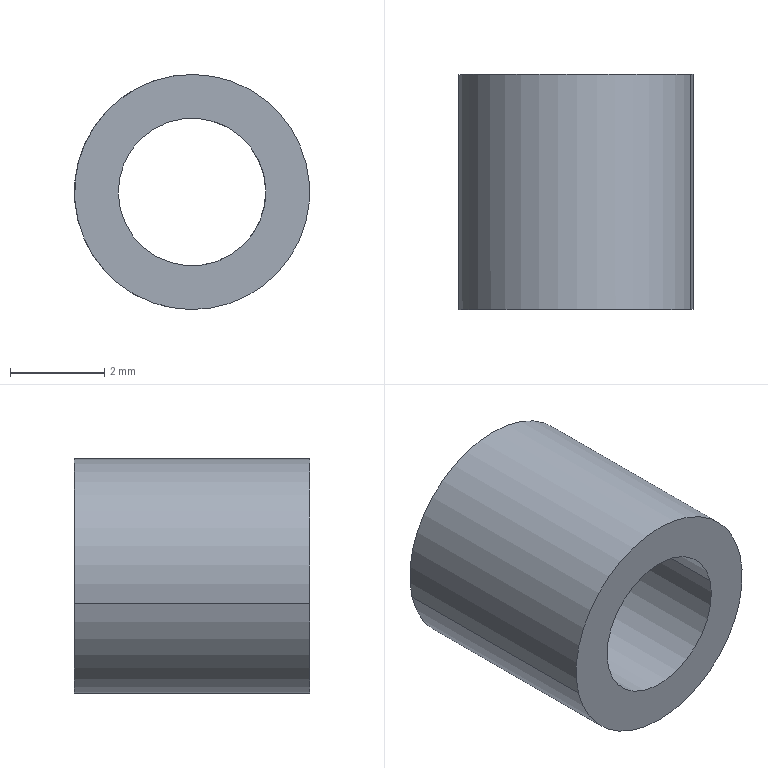Part | SolidWorks | features BaseBody 1 | 1 solid | 6 faces | box 5.005 x 5.005 x 5 mm | volume 59.456 mm3 | cylinder 4 | plane 2 | commonest cylinder face diameters 3.14 x2 5 x2
STEP:
#1=CARTESIAN_POINT('',(343.446,427.466,107.288));
#2=VERTEX_POINT('',#1);
#3=CARTESIAN_POINT('',(340.393,427.463,106.551));
#4=VERTEX_POINT('',#3);
#5=CARTESIAN_POINT('',(341.92,427.464,106.919));
#6=DIRECTION('',(0.0009599,-1.,0.));
#7=DIRECTION('',(-0.9721,-0.0009331,-0.2347));
#8=AXIS2_PLACEMENT_3D('',#5,#6,#7);
#9=CIRCLE('',#8,1.57);
#10=EDGE_CURVE('',#2,#4,#9,.T.);
#11=ORIENTED_EDGE('',*,*,#10,.F.);
#12=CARTESIAN_POINT('',(343.451,422.466,107.288));
#13=VERTEX_POINT('',#12);
#14=CARTESIAN_POINT('',(343.446,427.466,107.288));
#15=DIRECTION('',(0.0009599,-1.,0.));
#16=VECTOR('',#15,1000.);
#17=LINE('',#14,#16);
#18=EDGE_CURVE('',#2,#13,#17,.T.);
#19=ORIENTED_EDGE('',*,*,#18,.T.);
#20=CARTESIAN_POINT('',(340.398,422.463,106.551));
#21=VERTEX_POINT('',#20);
#22=CARTESIAN_POINT('',(341.924,422.464,106.919));
#23=DIRECTION('',(-0.0009599,1.,0.));
#24=DIRECTION('',(0.9721,0.0009331,0.2347));
#25=AXIS2_PLACEMENT_3D('',#22,#23,#24);
#26=CIRCLE('',#25,1.57);
#27=EDGE_CURVE('',#21,#13,#26,.T.);
#28=ORIENTED_EDGE('',*,*,#27,.F.);
#29=CARTESIAN_POINT('',(340.393,427.463,106.551));
#30=DIRECTION('',(0.0009599,-1.,0.));
#31=VECTOR('',#30,1000.);
#32=LINE('',#29,#31);
#33=EDGE_CURVE('',#4,#21,#32,.T.);
#34=ORIENTED_EDGE('',*,*,#33,.F.);
#35=EDGE_LOOP('',(#11,#19,#28,#34));
#36=FACE_OUTER_BOUND('',#35,.T.);
#37=CARTESIAN_POINT('',(341.92,427.464,106.919));
#38=DIRECTION('',(0.0009599,-1.,0.));
#39=DIRECTION('',(-0.9721,-0.0009331,-0.2347));
#40=AXIS2_PLACEMENT_3D('',#37,#38,#39);
#41=CYLINDRICAL_SURFACE('',#40,1.57);
#42=ADVANCED_FACE('',(#36),#41,.F.);
#43=CARTESIAN_POINT('',(344.35,427.466,107.506));
#44=VERTEX_POINT('',#43);
#45=CARTESIAN_POINT('',(339.489,427.462,106.332));
#46=VERTEX_POINT('',#45);
#47=CARTESIAN_POINT('',(341.92,427.464,106.919));
#48=DIRECTION('',(-0.0009599,1.,0.));
#49=DIRECTION('',(0.9721,0.0009331,0.2347));
#50=AXIS2_PLACEMENT_3D('',#47,#48,#49);
#51=CIRCLE('',#50,2.5);
#52=EDGE_CURVE('',#44,#46,#51,.T.);
#53=ORIENTED_EDGE('',*,*,#52,.F.);
#54=CARTESIAN_POINT('',(344.355,422.466,107.506));
#55=VERTEX_POINT('',#54);
#56=CARTESIAN_POINT('',(344.35,427.466,107.506));
#57=DIRECTION('',(0.0009599,-1.,0.));
#58=VECTOR('',#57,1000.);
#59=LINE('',#56,#58);
#60=EDGE_CURVE('',#44,#55,#59,.T.);
#61=ORIENTED_EDGE('',*,*,#60,.T.);
#62=CARTESIAN_POINT('',(339.494,422.462,106.332));
#63=VERTEX_POINT('',#62);
#64=CARTESIAN_POINT('',(341.924,422.464,106.919));
#65=DIRECTION('',(0.0009599,-1.,0.));
#66=DIRECTION('',(0.9721,0.0009331,0.2347));
#67=AXIS2_PLACEMENT_3D('',#64,#65,#66);
#68=CIRCLE('',#67,2.5);
#69=EDGE_CURVE('',#63,#55,#68,.T.);
#70=ORIENTED_EDGE('',*,*,#69,.F.);
#71=CARTESIAN_POINT('',(339.489,427.462,106.332));
#72=DIRECTION('',(0.0009599,-1.,0.));
#73=VECTOR('',#72,1000.);
#74=LINE('',#71,#73);
#75=EDGE_CURVE('',#46,#63,#74,.T.);
#76=ORIENTED_EDGE('',*,*,#75,.F.);
#77=EDGE_LOOP('',(#53,#61,#70,#76));
#78=FACE_OUTER_BOUND('',#77,.T.);
#79=CARTESIAN_POINT('',(341.92,427.464,106.919));
#80=DIRECTION('',(0.0009599,-1.,0.));
#81=DIRECTION('',(-0.9721,-0.0009331,-0.2347));
#82=AXIS2_PLACEMENT_3D('',#79,#80,#81);
#83=CYLINDRICAL_SURFACE('',#82,2.5);
#84=ADVANCED_FACE('',(#78),#83,.T.);
#85=ORIENTED_EDGE('',*,*,#27,.T.);
#86=CARTESIAN_POINT('',(341.924,422.464,106.919));
#87=DIRECTION('',(-0.0009599,1.,0.));
#88=DIRECTION('',(0.9721,0.0009331,0.2347));
#89=AXIS2_PLACEMENT_3D('',#86,#87,#88);
#90=CIRCLE('',#89,1.57);
#91=EDGE_CURVE('',#13,#21,#90,.T.);
#92=ORIENTED_EDGE('',*,*,#91,.T.);
#93=EDGE_LOOP('',(#85,#92));
#94=FACE_BOUND('',#93,.T.);
#95=ORIENTED_EDGE('',*,*,#69,.T.);
#96=CARTESIAN_POINT('',(341.924,422.464,106.919));
#97=DIRECTION('',(0.0009599,-1.,0.));
#98=DIRECTION('',(0.9721,0.0009331,0.2347));
#99=AXIS2_PLACEMENT_3D('',#96,#97,#98);
#100=CIRCLE('',#99,2.5);
#101=EDGE_CURVE('',#55,#63,#100,.T.);
#102=ORIENTED_EDGE('',*,*,#101,.T.);
#103=EDGE_LOOP('',(#95,#102));
#104=FACE_OUTER_BOUND('',#103,.T.);
#105=CARTESIAN_POINT('',(341.924,422.464,106.919));
#106=DIRECTION('',(-0.0009599,1.,0.));
#107=DIRECTION('',(0.,0.,1.));
#108=AXIS2_PLACEMENT_3D('',#105,#106,#107);
#109=PLANE('',#108);
#110=ADVANCED_FACE('',(#94,#104),#109,.F.);
#111=ORIENTED_EDGE('',*,*,#60,.F.);
#112=CARTESIAN_POINT('',(341.92,427.464,106.919));
#113=DIRECTION('',(-0.0009599,1.,0.));
#114=DIRECTION('',(0.9721,0.0009331,0.2347));
#115=AXIS2_PLACEMENT_3D('',#112,#113,#114);
#116=CIRCLE('',#115,2.5);
#117=EDGE_CURVE('',#46,#44,#116,.T.);
#118=ORIENTED_EDGE('',*,*,#117,.F.);
#119=ORIENTED_EDGE('',*,*,#75,.T.);
#120=ORIENTED_EDGE('',*,*,#101,.F.);
#121=EDGE_LOOP('',(#111,#118,#119,#120));
#122=FACE_OUTER_BOUND('',#121,.T.);
#123=CARTESIAN_POINT('',(341.92,427.464,106.919));
#124=DIRECTION('',(0.0009599,-1.,0.));
#125=DIRECTION('',(-0.9721,-0.0009331,-0.2347));
#126=AXIS2_PLACEMENT_3D('',#123,#124,#125);
#127=CYLINDRICAL_SURFACE('',#126,2.5);
#128=ADVANCED_FACE('',(#122),#127,.T.);
#129=CARTESIAN_POINT('',(341.92,427.464,106.919));
#130=DIRECTION('',(0.0009599,-1.,0.));
#131=DIRECTION('',(-0.9721,-0.0009331,-0.2347));
#132=AXIS2_PLACEMENT_3D('',#129,#130,#131);
#133=CIRCLE('',#132,1.57);
#134=EDGE_CURVE('',#4,#2,#133,.T.);
#135=ORIENTED_EDGE('',*,*,#134,.T.);
#136=ORIENTED_EDGE('',*,*,#10,.T.);
#137=EDGE_LOOP('',(#135,#136));
#138=FACE_BOUND('',#137,.T.);
#139=ORIENTED_EDGE('',*,*,#117,.T.);
#140=ORIENTED_EDGE('',*,*,#52,.T.);
#141=EDGE_LOOP('',(#139,#140));
#142=FACE_OUTER_BOUND('',#141,.T.);
#143=CARTESIAN_POINT('',(341.92,427.464,106.919));
#144=DIRECTION('',(-0.0009599,1.,0.));
#145=DIRECTION('',(0.,0.,1.));
#146=AXIS2_PLACEMENT_3D('',#143,#144,#145);
#147=PLANE('',#146);
#148=ADVANCED_FACE('',(#138,#142),#147,.T.);
#149=ORIENTED_EDGE('',*,*,#18,.F.);
#150=ORIENTED_EDGE('',*,*,#134,.F.);
#151=ORIENTED_EDGE('',*,*,#33,.T.);
#152=ORIENTED_EDGE('',*,*,#91,.F.);
#153=EDGE_LOOP('',(#149,#150,#151,#152));
#154=FACE_OUTER_BOUND('',#153,.T.);
#155=CARTESIAN_POINT('',(341.92,427.464,106.919));
#156=DIRECTION('',(0.0009599,-1.,0.));
#157=DIRECTION('',(-0.9721,-0.0009331,-0.2347));
#158=AXIS2_PLACEMENT_3D('',#155,#156,#157);
#159=CYLINDRICAL_SURFACE('',#158,1.57);
#160=ADVANCED_FACE('',(#154),#159,.F.);
#161=CLOSED_SHELL('',(#42,#84,#110,#128,#148,#160));
#162=MANIFOLD_SOLID_BREP('',#161);
#163=CARTESIAN_POINT('',(0.,0.,0.));
#164=DIRECTION('',(0.,0.,1.));
#165=DIRECTION('',(1.,0.,0.));
#166=AXIS2_PLACEMENT_3D('',#163,#164,#165);
#167=(LENGTH_UNIT()NAMED_UNIT(*)SI_UNIT(.MILLI.,.METRE.));
#168=UNCERTAINTY_MEASURE_WITH_UNIT(LENGTH_MEASURE(0.00001),#167,'','');
#169=(NAMED_UNIT(*)PLANE_ANGLE_UNIT()SI_UNIT($,.RADIAN.));
#170=(NAMED_UNIT(*)SI_UNIT($,.STERADIAN.)SOLID_ANGLE_UNIT());
#171=(GEOMETRIC_REPRESENTATION_CONTEXT(3)GLOBAL_UNCERTAINTY_ASSIGNED_CONTEXT((#168))GLOBAL_UNIT_ASSIGNED_CONTEXT((#167,#169,#170))REPRESENTATION_CONTEXT('',''));
#172=ADVANCED_BREP_SHAPE_REPRESENTATION('',(#162,#166),#171);